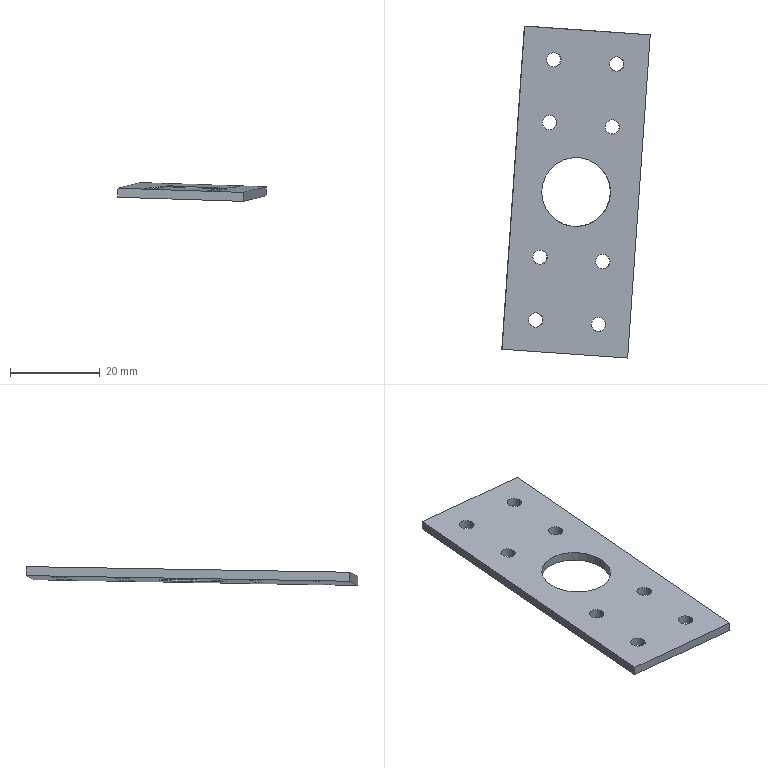Part | SolidWorks | features BaseBody 1 | 1 solid | 24 faces | box 33.003 x 73.785 x 4.177 mm | volume 3535 mm3 | cylinder 18 | plane 6 | commonest cylinder face diameters 3.2 x16 15.3 x2
STEP:
#1=CARTESIAN_POINT('',(-574.373,37.111,24.731));
#2=VERTEX_POINT('',#1);
#3=CARTESIAN_POINT('',(-571.174,37.111,24.63));
#4=VERTEX_POINT('',#3);
#5=CARTESIAN_POINT('',(-572.773,37.111,24.68));
#6=DIRECTION('',(0.03175,-0.01966,0.9993));
#7=DIRECTION('',(-0.9995,0.,0.03176));
#8=AXIS2_PLACEMENT_3D('',#5,#6,#7);
#9=CIRCLE('',#8,1.6);
#10=EDGE_CURVE('',#2,#4,#9,.T.);
#11=ORIENTED_EDGE('',*,*,#10,.T.);
#12=CARTESIAN_POINT('',(-571.238,37.15,22.631));
#13=VERTEX_POINT('',#12);
#14=CARTESIAN_POINT('',(-571.174,37.111,24.63));
#15=DIRECTION('',(-0.03175,0.01966,-0.9993));
#16=VECTOR('',#15,1000.);
#17=LINE('',#14,#16);
#18=EDGE_CURVE('',#4,#13,#17,.T.);
#19=ORIENTED_EDGE('',*,*,#18,.T.);
#20=CARTESIAN_POINT('',(-574.436,37.15,22.733));
#21=VERTEX_POINT('',#20);
#22=CARTESIAN_POINT('',(-572.837,37.15,22.682));
#23=DIRECTION('',(-0.03175,0.01966,-0.9993));
#24=DIRECTION('',(-0.9995,0.,0.03176));
#25=AXIS2_PLACEMENT_3D('',#22,#23,#24);
#26=CIRCLE('',#25,1.6);
#27=EDGE_CURVE('',#13,#21,#26,.T.);
#28=ORIENTED_EDGE('',*,*,#27,.T.);
#29=CARTESIAN_POINT('',(-574.373,37.111,24.731));
#30=DIRECTION('',(-0.03175,0.01966,-0.9993));
#31=VECTOR('',#30,1000.);
#32=LINE('',#29,#31);
#33=EDGE_CURVE('',#2,#21,#32,.T.);
#34=ORIENTED_EDGE('',*,*,#33,.F.);
#35=EDGE_LOOP('',(#11,#19,#28,#34));
#36=FACE_OUTER_BOUND('',#35,.T.);
#37=CARTESIAN_POINT('',(-572.773,37.111,24.68));
#38=DIRECTION('',(-0.03175,0.01966,-0.9993));
#39=DIRECTION('',(-0.9995,0.,0.03176));
#40=AXIS2_PLACEMENT_3D('',#37,#38,#39);
#41=CYLINDRICAL_SURFACE('',#40,1.6);
#42=ADVANCED_FACE('',(#36),#41,.F.);
#43=CARTESIAN_POINT('',(-572.151,23.147,24.386));
#44=VERTEX_POINT('',#43);
#45=CARTESIAN_POINT('',(-575.349,23.147,24.488));
#46=VERTEX_POINT('',#45);
#47=CARTESIAN_POINT('',(-573.75,23.147,24.437));
#48=DIRECTION('',(-0.03175,0.01966,-0.9993));
#49=DIRECTION('',(-0.9995,0.,0.03176));
#50=AXIS2_PLACEMENT_3D('',#47,#48,#49);
#51=CIRCLE('',#50,1.6);
#52=EDGE_CURVE('',#44,#46,#51,.T.);
#53=ORIENTED_EDGE('',*,*,#52,.F.);
#54=CARTESIAN_POINT('',(-572.214,23.186,22.387));
#55=VERTEX_POINT('',#54);
#56=CARTESIAN_POINT('',(-572.151,23.147,24.386));
#57=DIRECTION('',(-0.03175,0.01966,-0.9993));
#58=VECTOR('',#57,1000.);
#59=LINE('',#56,#58);
#60=EDGE_CURVE('',#44,#55,#59,.T.);
#61=ORIENTED_EDGE('',*,*,#60,.T.);
#62=CARTESIAN_POINT('',(-575.413,23.186,22.489));
#63=VERTEX_POINT('',#62);
#64=CARTESIAN_POINT('',(-573.813,23.186,22.438));
#65=DIRECTION('',(-0.03175,0.01966,-0.9993));
#66=DIRECTION('',(-0.9995,0.,0.03176));
#67=AXIS2_PLACEMENT_3D('',#64,#65,#66);
#68=CIRCLE('',#67,1.6);
#69=EDGE_CURVE('',#55,#63,#68,.T.);
#70=ORIENTED_EDGE('',*,*,#69,.T.);
#71=CARTESIAN_POINT('',(-575.349,23.147,24.488));
#72=DIRECTION('',(-0.03175,0.01966,-0.9993));
#73=VECTOR('',#72,1000.);
#74=LINE('',#71,#73);
#75=EDGE_CURVE('',#46,#63,#74,.T.);
#76=ORIENTED_EDGE('',*,*,#75,.F.);
#77=EDGE_LOOP('',(#53,#61,#70,#76));
#78=FACE_OUTER_BOUND('',#77,.T.);
#79=CARTESIAN_POINT('',(-573.75,23.147,24.437));
#80=DIRECTION('',(-0.03175,0.01966,-0.9993));
#81=DIRECTION('',(-0.9995,0.,0.03176));
#82=AXIS2_PLACEMENT_3D('',#79,#80,#81);
#83=CYLINDRICAL_SURFACE('',#82,1.6);
#84=ADVANCED_FACE('',(#78),#83,.F.);
#85=CARTESIAN_POINT('',(-555.123,66.061,24.689));
#86=VERTEX_POINT('',#85);
#87=CARTESIAN_POINT('',(-558.321,66.061,24.791));
#88=VERTEX_POINT('',#87);
#89=CARTESIAN_POINT('',(-556.722,66.061,24.74));
#90=DIRECTION('',(-0.03175,0.01966,-0.9993));
#91=DIRECTION('',(-0.9995,0.,0.03176));
#92=AXIS2_PLACEMENT_3D('',#89,#90,#91);
#93=CIRCLE('',#92,1.6);
#94=EDGE_CURVE('',#86,#88,#93,.T.);
#95=ORIENTED_EDGE('',*,*,#94,.F.);
#96=CARTESIAN_POINT('',(-555.186,66.1,22.691));
#97=VERTEX_POINT('',#96);
#98=CARTESIAN_POINT('',(-555.123,66.061,24.689));
#99=DIRECTION('',(-0.03175,0.01966,-0.9993));
#100=VECTOR('',#99,1000.);
#101=LINE('',#98,#100);
#102=EDGE_CURVE('',#86,#97,#101,.T.);
#103=ORIENTED_EDGE('',*,*,#102,.T.);
#104=CARTESIAN_POINT('',(-558.385,66.1,22.792));
#105=VERTEX_POINT('',#104);
#106=CARTESIAN_POINT('',(-556.786,66.1,22.741));
#107=DIRECTION('',(-0.03175,0.01966,-0.9993));
#108=DIRECTION('',(-0.9995,0.,0.03176));
#109=AXIS2_PLACEMENT_3D('',#106,#107,#108);
#110=CIRCLE('',#109,1.6);
#111=EDGE_CURVE('',#97,#105,#110,.T.);
#112=ORIENTED_EDGE('',*,*,#111,.T.);
#113=CARTESIAN_POINT('',(-558.321,66.061,24.791));
#114=DIRECTION('',(-0.03175,0.01966,-0.9993));
#115=VECTOR('',#114,1000.);
#116=LINE('',#113,#115);
#117=EDGE_CURVE('',#88,#105,#116,.T.);
#118=ORIENTED_EDGE('',*,*,#117,.F.);
#119=EDGE_LOOP('',(#95,#103,#112,#118));
#120=FACE_OUTER_BOUND('',#119,.T.);
#121=CARTESIAN_POINT('',(-556.722,66.061,24.74));
#122=DIRECTION('',(-0.03175,0.01966,-0.9993));
#123=DIRECTION('',(-0.9995,0.,0.03176));
#124=AXIS2_PLACEMENT_3D('',#121,#122,#123);
#125=CYLINDRICAL_SURFACE('',#124,1.6);
#126=ADVANCED_FACE('',(#120),#125,.F.);
#127=CARTESIAN_POINT('',(-569.082,67.029,25.152));
#128=VERTEX_POINT('',#127);
#129=CARTESIAN_POINT('',(-572.28,67.029,25.253));
#130=VERTEX_POINT('',#129);
#131=CARTESIAN_POINT('',(-570.681,67.029,25.203));
#132=DIRECTION('',(-0.03175,0.01966,-0.9993));
#133=DIRECTION('',(-0.9995,0.,0.03176));
#134=AXIS2_PLACEMENT_3D('',#131,#132,#133);
#135=CIRCLE('',#134,1.6);
#136=EDGE_CURVE('',#128,#130,#135,.T.);
#137=ORIENTED_EDGE('',*,*,#136,.F.);
#138=CARTESIAN_POINT('',(-569.145,67.068,23.153));
#139=VERTEX_POINT('',#138);
#140=CARTESIAN_POINT('',(-569.082,67.029,25.152));
#141=DIRECTION('',(-0.03175,0.01966,-0.9993));
#142=VECTOR('',#141,1000.);
#143=LINE('',#140,#142);
#144=EDGE_CURVE('',#128,#139,#143,.T.);
#145=ORIENTED_EDGE('',*,*,#144,.T.);
#146=CARTESIAN_POINT('',(-572.344,67.068,23.255));
#147=VERTEX_POINT('',#146);
#148=CARTESIAN_POINT('',(-570.745,67.068,23.204));
#149=DIRECTION('',(-0.03175,0.01966,-0.9993));
#150=DIRECTION('',(-0.9995,0.,0.03176));
#151=AXIS2_PLACEMENT_3D('',#148,#149,#150);
#152=CIRCLE('',#151,1.6);
#153=EDGE_CURVE('',#139,#147,#152,.T.);
#154=ORIENTED_EDGE('',*,*,#153,.T.);
#155=CARTESIAN_POINT('',(-572.28,67.029,25.253));
#156=DIRECTION('',(-0.03175,0.01966,-0.9993));
#157=VECTOR('',#156,1000.);
#158=LINE('',#155,#157);
#159=EDGE_CURVE('',#130,#147,#158,.T.);
#160=ORIENTED_EDGE('',*,*,#159,.F.);
#161=EDGE_LOOP('',(#137,#145,#154,#160));
#162=FACE_OUTER_BOUND('',#161,.T.);
#163=CARTESIAN_POINT('',(-570.681,67.029,25.203));
#164=DIRECTION('',(-0.03175,0.01966,-0.9993));
#165=DIRECTION('',(-0.9995,0.,0.03176));
#166=AXIS2_PLACEMENT_3D('',#163,#164,#165);
#167=CYLINDRICAL_SURFACE('',#166,1.6);
#168=ADVANCED_FACE('',(#162),#167,.F.);
#169=CARTESIAN_POINT('',(-568.105,80.992,25.396));
#170=VERTEX_POINT('',#169);
#171=CARTESIAN_POINT('',(-571.304,80.992,25.497));
#172=VERTEX_POINT('',#171);
#173=CARTESIAN_POINT('',(-569.704,80.992,25.446));
#174=DIRECTION('',(-0.03175,0.01966,-0.9993));
#175=DIRECTION('',(-0.9995,0.,0.03176));
#176=AXIS2_PLACEMENT_3D('',#173,#174,#175);
#177=CIRCLE('',#176,1.6);
#178=EDGE_CURVE('',#170,#172,#177,.T.);
#179=ORIENTED_EDGE('',*,*,#178,.F.);
#180=CARTESIAN_POINT('',(-568.169,81.032,23.397));
#181=VERTEX_POINT('',#180);
#182=CARTESIAN_POINT('',(-568.105,80.992,25.396));
#183=DIRECTION('',(-0.03175,0.01966,-0.9993));
#184=VECTOR('',#183,1000.);
#185=LINE('',#182,#184);
#186=EDGE_CURVE('',#170,#181,#185,.T.);
#187=ORIENTED_EDGE('',*,*,#186,.T.);
#188=CARTESIAN_POINT('',(-571.367,81.032,23.499));
#189=VERTEX_POINT('',#188);
#190=CARTESIAN_POINT('',(-569.768,81.032,23.448));
#191=DIRECTION('',(-0.03175,0.01966,-0.9993));
#192=DIRECTION('',(-0.9995,0.,0.03176));
#193=AXIS2_PLACEMENT_3D('',#190,#191,#192);
#194=CIRCLE('',#193,1.6);
#195=EDGE_CURVE('',#181,#189,#194,.T.);
#196=ORIENTED_EDGE('',*,*,#195,.T.);
#197=CARTESIAN_POINT('',(-571.304,80.992,25.497));
#198=DIRECTION('',(-0.03175,0.01966,-0.9993));
#199=VECTOR('',#198,1000.);
#200=LINE('',#197,#199);
#201=EDGE_CURVE('',#172,#189,#200,.T.);
#202=ORIENTED_EDGE('',*,*,#201,.F.);
#203=EDGE_LOOP('',(#179,#187,#196,#202));
#204=FACE_OUTER_BOUND('',#203,.T.);
#205=CARTESIAN_POINT('',(-569.704,80.992,25.446));
#206=DIRECTION('',(-0.03175,0.01966,-0.9993));
#207=DIRECTION('',(-0.9995,0.,0.03176));
#208=AXIS2_PLACEMENT_3D('',#205,#206,#207);
#209=CYLINDRICAL_SURFACE('',#208,1.6);
#210=ADVANCED_FACE('',(#204),#209,.F.);
#211=CARTESIAN_POINT('',(-554.146,80.024,24.933));
#212=VERTEX_POINT('',#211);
#213=CARTESIAN_POINT('',(-557.345,80.024,25.035));
#214=VERTEX_POINT('',#213);
#215=CARTESIAN_POINT('',(-555.746,80.024,24.984));
#216=DIRECTION('',(-0.03175,0.01966,-0.9993));
#217=DIRECTION('',(-0.9995,0.,0.03176));
#218=AXIS2_PLACEMENT_3D('',#215,#216,#217);
#219=CIRCLE('',#218,1.6);
#220=EDGE_CURVE('',#212,#214,#219,.T.);
#221=ORIENTED_EDGE('',*,*,#220,.F.);
#222=CARTESIAN_POINT('',(-554.21,80.064,22.934));
#223=VERTEX_POINT('',#222);
#224=CARTESIAN_POINT('',(-554.146,80.024,24.933));
#225=DIRECTION('',(-0.03175,0.01966,-0.9993));
#226=VECTOR('',#225,1000.);
#227=LINE('',#224,#226);
#228=EDGE_CURVE('',#212,#223,#227,.T.);
#229=ORIENTED_EDGE('',*,*,#228,.T.);
#230=CARTESIAN_POINT('',(-557.408,80.064,23.036));
#231=VERTEX_POINT('',#230);
#232=CARTESIAN_POINT('',(-555.809,80.064,22.985));
#233=DIRECTION('',(-0.03175,0.01966,-0.9993));
#234=DIRECTION('',(-0.9995,0.,0.03176));
#235=AXIS2_PLACEMENT_3D('',#232,#233,#234);
#236=CIRCLE('',#235,1.6);
#237=EDGE_CURVE('',#223,#231,#236,.T.);
#238=ORIENTED_EDGE('',*,*,#237,.T.);
#239=CARTESIAN_POINT('',(-557.345,80.024,25.035));
#240=DIRECTION('',(-0.03175,0.01966,-0.9993));
#241=VECTOR('',#240,1000.);
#242=LINE('',#239,#241);
#243=EDGE_CURVE('',#214,#231,#242,.T.);
#244=ORIENTED_EDGE('',*,*,#243,.F.);
#245=EDGE_LOOP('',(#221,#229,#238,#244));
#246=FACE_OUTER_BOUND('',#245,.T.);
#247=CARTESIAN_POINT('',(-555.746,80.024,24.984));
#248=DIRECTION('',(-0.03175,0.01966,-0.9993));
#249=DIRECTION('',(-0.9995,0.,0.03176));
#250=AXIS2_PLACEMENT_3D('',#247,#248,#249);
#251=CYLINDRICAL_SURFACE('',#250,1.6);
#252=ADVANCED_FACE('',(#246),#251,.F.);
#253=CARTESIAN_POINT('',(-557.102,51.586,24.467));
#254=VERTEX_POINT('',#253);
#255=CARTESIAN_POINT('',(-572.394,51.586,24.953));
#256=VERTEX_POINT('',#255);
#257=CARTESIAN_POINT('',(-564.748,51.586,24.71));
#258=DIRECTION('',(-0.03175,0.01966,-0.9993));
#259=DIRECTION('',(-0.9995,0.,0.03176));
#260=AXIS2_PLACEMENT_3D('',#257,#258,#259);
#261=CIRCLE('',#260,7.65);
#262=EDGE_CURVE('',#254,#256,#261,.T.);
#263=ORIENTED_EDGE('',*,*,#262,.F.);
#264=CARTESIAN_POINT('',(-557.165,51.625,22.469));
#265=VERTEX_POINT('',#264);
#266=CARTESIAN_POINT('',(-557.102,51.586,24.467));
#267=DIRECTION('',(-0.03175,0.01966,-0.9993));
#268=VECTOR('',#267,1000.);
#269=LINE('',#266,#268);
#270=EDGE_CURVE('',#254,#265,#269,.T.);
#271=ORIENTED_EDGE('',*,*,#270,.T.);
#272=CARTESIAN_POINT('',(-572.457,51.625,22.955));
#273=VERTEX_POINT('',#272);
#274=CARTESIAN_POINT('',(-564.811,51.625,22.712));
#275=DIRECTION('',(-0.03175,0.01966,-0.9993));
#276=DIRECTION('',(-0.9995,0.,0.03176));
#277=AXIS2_PLACEMENT_3D('',#274,#275,#276);
#278=CIRCLE('',#277,7.65);
#279=EDGE_CURVE('',#265,#273,#278,.T.);
#280=ORIENTED_EDGE('',*,*,#279,.T.);
#281=CARTESIAN_POINT('',(-572.394,51.586,24.953));
#282=DIRECTION('',(-0.03175,0.01966,-0.9993));
#283=VECTOR('',#282,1000.);
#284=LINE('',#281,#283);
#285=EDGE_CURVE('',#256,#273,#284,.T.);
#286=ORIENTED_EDGE('',*,*,#285,.F.);
#287=EDGE_LOOP('',(#263,#271,#280,#286));
#288=FACE_OUTER_BOUND('',#287,.T.);
#289=CARTESIAN_POINT('',(-564.748,51.586,24.71));
#290=DIRECTION('',(-0.03175,0.01966,-0.9993));
#291=DIRECTION('',(-0.9995,0.,0.03176));
#292=AXIS2_PLACEMENT_3D('',#289,#290,#291);
#293=CYLINDRICAL_SURFACE('',#292,7.65);
#294=ADVANCED_FACE('',(#288),#293,.F.);
#295=CARTESIAN_POINT('',(-558.192,22.179,23.923));
#296=VERTEX_POINT('',#295);
#297=CARTESIAN_POINT('',(-561.39,22.179,24.025));
#298=VERTEX_POINT('',#297);
#299=CARTESIAN_POINT('',(-559.791,22.179,23.974));
#300=DIRECTION('',(-0.03175,0.01966,-0.9993));
#301=DIRECTION('',(-0.9995,0.,0.03176));
#302=AXIS2_PLACEMENT_3D('',#299,#300,#301);
#303=CIRCLE('',#302,1.6);
#304=EDGE_CURVE('',#296,#298,#303,.T.);
#305=ORIENTED_EDGE('',*,*,#304,.F.);
#306=CARTESIAN_POINT('',(-558.255,22.218,21.925));
#307=VERTEX_POINT('',#306);
#308=CARTESIAN_POINT('',(-558.192,22.179,23.923));
#309=DIRECTION('',(-0.03175,0.01966,-0.9993));
#310=VECTOR('',#309,1000.);
#311=LINE('',#308,#310);
#312=EDGE_CURVE('',#296,#307,#311,.T.);
#313=ORIENTED_EDGE('',*,*,#312,.T.);
#314=CARTESIAN_POINT('',(-561.454,22.218,22.026));
#315=VERTEX_POINT('',#314);
#316=CARTESIAN_POINT('',(-559.855,22.218,21.976));
#317=DIRECTION('',(-0.03175,0.01966,-0.9993));
#318=DIRECTION('',(-0.9995,0.,0.03176));
#319=AXIS2_PLACEMENT_3D('',#316,#317,#318);
#320=CIRCLE('',#319,1.6);
#321=EDGE_CURVE('',#307,#315,#320,.T.);
#322=ORIENTED_EDGE('',*,*,#321,.T.);
#323=CARTESIAN_POINT('',(-561.39,22.179,24.025));
#324=DIRECTION('',(-0.03175,0.01966,-0.9993));
#325=VECTOR('',#324,1000.);
#326=LINE('',#323,#325);
#327=EDGE_CURVE('',#298,#315,#326,.T.);
#328=ORIENTED_EDGE('',*,*,#327,.F.);
#329=EDGE_LOOP('',(#305,#313,#322,#328));
#330=FACE_OUTER_BOUND('',#329,.T.);
#331=CARTESIAN_POINT('',(-559.791,22.179,23.974));
#332=DIRECTION('',(-0.03175,0.01966,-0.9993));
#333=DIRECTION('',(-0.9995,0.,0.03176));
#334=AXIS2_PLACEMENT_3D('',#331,#332,#333);
#335=CYLINDRICAL_SURFACE('',#334,1.6);
#336=ADVANCED_FACE('',(#330),#335,.F.);
#337=CARTESIAN_POINT('',(-557.215,36.143,24.167));
#338=VERTEX_POINT('',#337);
#339=CARTESIAN_POINT('',(-560.414,36.143,24.269));
#340=VERTEX_POINT('',#339);
#341=CARTESIAN_POINT('',(-558.815,36.143,24.218));
#342=DIRECTION('',(-0.03175,0.01966,-0.9993));
#343=DIRECTION('',(-0.9995,0.,0.03176));
#344=AXIS2_PLACEMENT_3D('',#341,#342,#343);
#345=CIRCLE('',#344,1.6);
#346=EDGE_CURVE('',#338,#340,#345,.T.);
#347=ORIENTED_EDGE('',*,*,#346,.F.);
#348=CARTESIAN_POINT('',(-557.279,36.182,22.168));
#349=VERTEX_POINT('',#348);
#350=CARTESIAN_POINT('',(-557.215,36.143,24.167));
#351=DIRECTION('',(-0.03175,0.01966,-0.9993));
#352=VECTOR('',#351,1000.);
#353=LINE('',#350,#352);
#354=EDGE_CURVE('',#338,#349,#353,.T.);
#355=ORIENTED_EDGE('',*,*,#354,.T.);
#356=CARTESIAN_POINT('',(-560.477,36.182,22.27));
#357=VERTEX_POINT('',#356);
#358=CARTESIAN_POINT('',(-558.878,36.182,22.219));
#359=DIRECTION('',(-0.03175,0.01966,-0.9993));
#360=DIRECTION('',(-0.9995,0.,0.03176));
#361=AXIS2_PLACEMENT_3D('',#358,#359,#360);
#362=CIRCLE('',#361,1.6);
#363=EDGE_CURVE('',#349,#357,#362,.T.);
#364=ORIENTED_EDGE('',*,*,#363,.T.);
#365=CARTESIAN_POINT('',(-560.414,36.143,24.269));
#366=DIRECTION('',(-0.03175,0.01966,-0.9993));
#367=VECTOR('',#366,1000.);
#368=LINE('',#365,#367);
#369=EDGE_CURVE('',#340,#357,#368,.T.);
#370=ORIENTED_EDGE('',*,*,#369,.F.);
#371=EDGE_LOOP('',(#347,#355,#364,#370));
#372=FACE_OUTER_BOUND('',#371,.T.);
#373=CARTESIAN_POINT('',(-558.815,36.143,24.218));
#374=DIRECTION('',(-0.03175,0.01966,-0.9993));
#375=DIRECTION('',(-0.9995,0.,0.03176));
#376=AXIS2_PLACEMENT_3D('',#373,#374,#375);
#377=CYLINDRICAL_SURFACE('',#376,1.6);
#378=ADVANCED_FACE('',(#372),#377,.F.);
#379=ORIENTED_EDGE('',*,*,#18,.F.);
#380=CARTESIAN_POINT('',(-572.773,37.111,24.68));
#381=DIRECTION('',(0.03175,-0.01966,0.9993));
#382=DIRECTION('',(-0.9995,0.,0.03176));
#383=AXIS2_PLACEMENT_3D('',#380,#381,#382);
#384=CIRCLE('',#383,1.6);
#385=EDGE_CURVE('',#4,#2,#384,.T.);
#386=ORIENTED_EDGE('',*,*,#385,.T.);
#387=ORIENTED_EDGE('',*,*,#33,.T.);
#388=CARTESIAN_POINT('',(-572.837,37.15,22.682));
#389=DIRECTION('',(-0.03175,0.01966,-0.9993));
#390=DIRECTION('',(-0.9995,0.,0.03176));
#391=AXIS2_PLACEMENT_3D('',#388,#389,#390);
#392=CIRCLE('',#391,1.6);
#393=EDGE_CURVE('',#21,#13,#392,.T.);
#394=ORIENTED_EDGE('',*,*,#393,.T.);
#395=EDGE_LOOP('',(#379,#386,#387,#394));
#396=FACE_OUTER_BOUND('',#395,.T.);
#397=CARTESIAN_POINT('',(-572.773,37.111,24.68));
#398=DIRECTION('',(-0.03175,0.01966,-0.9993));
#399=DIRECTION('',(-0.9995,0.,0.03176));
#400=AXIS2_PLACEMENT_3D('',#397,#398,#399);
#401=CYLINDRICAL_SURFACE('',#400,1.6);
#402=ADVANCED_FACE('',(#396),#401,.F.);
#403=ORIENTED_EDGE('',*,*,#393,.F.);
#404=ORIENTED_EDGE('',*,*,#27,.F.);
#405=EDGE_LOOP('',(#403,#404));
#406=FACE_BOUND('',#405,.T.);
#407=CARTESIAN_POINT('',(-573.813,23.186,22.438));
#408=DIRECTION('',(-0.03175,0.01966,-0.9993));
#409=DIRECTION('',(-0.9995,0.,0.03176));
#410=AXIS2_PLACEMENT_3D('',#407,#408,#409);
#411=CIRCLE('',#410,1.6);
#412=EDGE_CURVE('',#63,#55,#411,.T.);
#413=ORIENTED_EDGE('',*,*,#412,.F.);
#414=ORIENTED_EDGE('',*,*,#69,.F.);
#415=EDGE_LOOP('',(#413,#414));
#416=FACE_BOUND('',#415,.T.);
#417=CARTESIAN_POINT('',(-556.786,66.1,22.741));
#418=DIRECTION('',(-0.03175,0.01966,-0.9993));
#419=DIRECTION('',(-0.9995,0.,0.03176));
#420=AXIS2_PLACEMENT_3D('',#417,#418,#419);
#421=CIRCLE('',#420,1.6);
#422=EDGE_CURVE('',#105,#97,#421,.T.);
#423=ORIENTED_EDGE('',*,*,#422,.F.);
#424=ORIENTED_EDGE('',*,*,#111,.F.);
#425=EDGE_LOOP('',(#423,#424));
#426=FACE_BOUND('',#425,.T.);
#427=CARTESIAN_POINT('',(-570.745,67.068,23.204));
#428=DIRECTION('',(-0.03175,0.01966,-0.9993));
#429=DIRECTION('',(-0.9995,0.,0.03176));
#430=AXIS2_PLACEMENT_3D('',#427,#428,#429);
#431=CIRCLE('',#430,1.6);
#432=EDGE_CURVE('',#147,#139,#431,.T.);
#433=ORIENTED_EDGE('',*,*,#432,.F.);
#434=ORIENTED_EDGE('',*,*,#153,.F.);
#435=EDGE_LOOP('',(#433,#434));
#436=FACE_BOUND('',#435,.T.);
#437=CARTESIAN_POINT('',(-569.768,81.032,23.448));
#438=DIRECTION('',(-0.03175,0.01966,-0.9993));
#439=DIRECTION('',(-0.9995,0.,0.03176));
#440=AXIS2_PLACEMENT_3D('',#437,#438,#439);
#441=CIRCLE('',#440,1.6);
#442=EDGE_CURVE('',#189,#181,#441,.T.);
#443=ORIENTED_EDGE('',*,*,#442,.F.);
#444=ORIENTED_EDGE('',*,*,#195,.F.);
#445=EDGE_LOOP('',(#443,#444));
#446=FACE_BOUND('',#445,.T.);
#447=CARTESIAN_POINT('',(-555.809,80.064,22.985));
#448=DIRECTION('',(-0.03175,0.01966,-0.9993));
#449=DIRECTION('',(-0.9995,0.,0.03176));
#450=AXIS2_PLACEMENT_3D('',#447,#448,#449);
#451=CIRCLE('',#450,1.6);
#452=EDGE_CURVE('',#231,#223,#451,.T.);
#453=ORIENTED_EDGE('',*,*,#452,.F.);
#454=ORIENTED_EDGE('',*,*,#237,.F.);
#455=EDGE_LOOP('',(#453,#454));
#456=FACE_BOUND('',#455,.T.);
#457=CARTESIAN_POINT('',(-564.811,51.625,22.712));
#458=DIRECTION('',(-0.03175,0.01966,-0.9993));
#459=DIRECTION('',(-0.9995,0.,0.03176));
#460=AXIS2_PLACEMENT_3D('',#457,#458,#459);
#461=CIRCLE('',#460,7.65);
#462=EDGE_CURVE('',#273,#265,#461,.T.);
#463=ORIENTED_EDGE('',*,*,#462,.F.);
#464=ORIENTED_EDGE('',*,*,#279,.F.);
#465=EDGE_LOOP('',(#463,#464));
#466=FACE_BOUND('',#465,.T.);
#467=CARTESIAN_POINT('',(-559.855,22.218,21.976));
#468=DIRECTION('',(-0.03175,0.01966,-0.9993));
#469=DIRECTION('',(-0.9995,0.,0.03176));
#470=AXIS2_PLACEMENT_3D('',#467,#468,#469);
#471=CIRCLE('',#470,1.6);
#472=EDGE_CURVE('',#315,#307,#471,.T.);
#473=ORIENTED_EDGE('',*,*,#472,.F.);
#474=ORIENTED_EDGE('',*,*,#321,.F.);
#475=EDGE_LOOP('',(#473,#474));
#476=FACE_BOUND('',#475,.T.);
#477=CARTESIAN_POINT('',(-558.878,36.182,22.219));
#478=DIRECTION('',(-0.03175,0.01966,-0.9993));
#479=DIRECTION('',(-0.9995,0.,0.03176));
#480=AXIS2_PLACEMENT_3D('',#477,#478,#479);
#481=CIRCLE('',#480,1.6);
#482=EDGE_CURVE('',#357,#349,#481,.T.);
#483=ORIENTED_EDGE('',*,*,#482,.F.);
#484=ORIENTED_EDGE('',*,*,#363,.F.);
#485=EDGE_LOOP('',(#483,#484));
#486=FACE_BOUND('',#485,.T.);
#487=CARTESIAN_POINT('',(-548.341,86.561,22.876));
#488=VERTEX_POINT('',#487);
#489=CARTESIAN_POINT('',(-576.259,88.498,23.801));
#490=VERTEX_POINT('',#489);
#491=CARTESIAN_POINT('',(-548.341,86.561,22.876));
#492=DIRECTION('',(-0.9971,0.06916,0.03304));
#493=VECTOR('',#492,1000.);
#494=LINE('',#491,#493);
#495=EDGE_CURVE('',#488,#490,#494,.T.);
#496=ORIENTED_EDGE('',*,*,#495,.F.);
#497=CARTESIAN_POINT('',(-553.364,14.752,21.622));
#498=VERTEX_POINT('',#497);
#499=CARTESIAN_POINT('',(-553.364,14.752,21.622));
#500=DIRECTION('',(0.06976,0.9974,0.01741));
#501=VECTOR('',#500,1000.);
#502=LINE('',#499,#501);
#503=EDGE_CURVE('',#498,#488,#502,.T.);
#504=ORIENTED_EDGE('',*,*,#503,.F.);
#505=CARTESIAN_POINT('',(-581.281,16.689,22.548));
#506=VERTEX_POINT('',#505);
#507=CARTESIAN_POINT('',(-581.281,16.689,22.548));
#508=DIRECTION('',(0.9971,-0.06916,-0.03304));
#509=VECTOR('',#508,1000.);
#510=LINE('',#507,#509);
#511=EDGE_CURVE('',#506,#498,#510,.T.);
#512=ORIENTED_EDGE('',*,*,#511,.F.);
#513=CARTESIAN_POINT('',(-576.259,88.498,23.801));
#514=DIRECTION('',(-0.06976,-0.9974,-0.01741));
#515=VECTOR('',#514,1000.);
#516=LINE('',#513,#515);
#517=EDGE_CURVE('',#490,#506,#516,.T.);
#518=ORIENTED_EDGE('',*,*,#517,.F.);
#519=EDGE_LOOP('',(#496,#504,#512,#518));
#520=FACE_OUTER_BOUND('',#519,.T.);
#521=CARTESIAN_POINT('',(-581.48,14.31,22.507));
#522=DIRECTION('',(0.03175,-0.01966,0.9993));
#523=DIRECTION('',(0.9995,0.,-0.03176));
#524=AXIS2_PLACEMENT_3D('',#521,#522,#523);
#525=PLANE('',#524);
#526=ADVANCED_FACE('',(#406,#416,#426,#436,#446,#456,#466,#476,#486,#520),#525,.F.);
#527=ORIENTED_EDGE('',*,*,#10,.F.);
#528=ORIENTED_EDGE('',*,*,#385,.F.);
#529=EDGE_LOOP('',(#527,#528));
#530=FACE_BOUND('',#529,.T.);
#531=CARTESIAN_POINT('',(-573.75,23.147,24.437));
#532=DIRECTION('',(-0.03175,0.01966,-0.9993));
#533=DIRECTION('',(-0.9995,0.,0.03176));
#534=AXIS2_PLACEMENT_3D('',#531,#532,#533);
#535=CIRCLE('',#534,1.6);
#536=EDGE_CURVE('',#46,#44,#535,.T.);
#537=ORIENTED_EDGE('',*,*,#536,.T.);
#538=ORIENTED_EDGE('',*,*,#52,.T.);
#539=EDGE_LOOP('',(#537,#538));
#540=FACE_BOUND('',#539,.T.);
#541=CARTESIAN_POINT('',(-556.722,66.061,24.74));
#542=DIRECTION('',(-0.03175,0.01966,-0.9993));
#543=DIRECTION('',(-0.9995,0.,0.03176));
#544=AXIS2_PLACEMENT_3D('',#541,#542,#543);
#545=CIRCLE('',#544,1.6);
#546=EDGE_CURVE('',#88,#86,#545,.T.);
#547=ORIENTED_EDGE('',*,*,#546,.T.);
#548=ORIENTED_EDGE('',*,*,#94,.T.);
#549=EDGE_LOOP('',(#547,#548));
#550=FACE_BOUND('',#549,.T.);
#551=CARTESIAN_POINT('',(-570.681,67.029,25.203));
#552=DIRECTION('',(-0.03175,0.01966,-0.9993));
#553=DIRECTION('',(-0.9995,0.,0.03176));
#554=AXIS2_PLACEMENT_3D('',#551,#552,#553);
#555=CIRCLE('',#554,1.6);
#556=EDGE_CURVE('',#130,#128,#555,.T.);
#557=ORIENTED_EDGE('',*,*,#556,.T.);
#558=ORIENTED_EDGE('',*,*,#136,.T.);
#559=EDGE_LOOP('',(#557,#558));
#560=FACE_BOUND('',#559,.T.);
#561=CARTESIAN_POINT('',(-569.704,80.992,25.446));
#562=DIRECTION('',(-0.03175,0.01966,-0.9993));
#563=DIRECTION('',(-0.9995,0.,0.03176));
#564=AXIS2_PLACEMENT_3D('',#561,#562,#563);
#565=CIRCLE('',#564,1.6);
#566=EDGE_CURVE('',#172,#170,#565,.T.);
#567=ORIENTED_EDGE('',*,*,#566,.T.);
#568=ORIENTED_EDGE('',*,*,#178,.T.);
#569=EDGE_LOOP('',(#567,#568));
#570=FACE_BOUND('',#569,.T.);
#571=CARTESIAN_POINT('',(-555.746,80.024,24.984));
#572=DIRECTION('',(-0.03175,0.01966,-0.9993));
#573=DIRECTION('',(-0.9995,0.,0.03176));
#574=AXIS2_PLACEMENT_3D('',#571,#572,#573);
#575=CIRCLE('',#574,1.6);
#576=EDGE_CURVE('',#214,#212,#575,.T.);
#577=ORIENTED_EDGE('',*,*,#576,.T.);
#578=ORIENTED_EDGE('',*,*,#220,.T.);
#579=EDGE_LOOP('',(#577,#578));
#580=FACE_BOUND('',#579,.T.);
#581=CARTESIAN_POINT('',(-564.748,51.586,24.71));
#582=DIRECTION('',(-0.03175,0.01966,-0.9993));
#583=DIRECTION('',(-0.9995,0.,0.03176));
#584=AXIS2_PLACEMENT_3D('',#581,#582,#583);
#585=CIRCLE('',#584,7.65);
#586=EDGE_CURVE('',#256,#254,#585,.T.);
#587=ORIENTED_EDGE('',*,*,#586,.T.);
#588=ORIENTED_EDGE('',*,*,#262,.T.);
#589=EDGE_LOOP('',(#587,#588));
#590=FACE_BOUND('',#589,.T.);
#591=CARTESIAN_POINT('',(-559.791,22.179,23.974));
#592=DIRECTION('',(-0.03175,0.01966,-0.9993));
#593=DIRECTION('',(-0.9995,0.,0.03176));
#594=AXIS2_PLACEMENT_3D('',#591,#592,#593);
#595=CIRCLE('',#594,1.6);
#596=EDGE_CURVE('',#298,#296,#595,.T.);
#597=ORIENTED_EDGE('',*,*,#596,.T.);
#598=ORIENTED_EDGE('',*,*,#304,.T.);
#599=EDGE_LOOP('',(#597,#598));
#600=FACE_BOUND('',#599,.T.);
#601=CARTESIAN_POINT('',(-558.815,36.143,24.218));
#602=DIRECTION('',(-0.03175,0.01966,-0.9993));
#603=DIRECTION('',(-0.9995,0.,0.03176));
#604=AXIS2_PLACEMENT_3D('',#601,#602,#603);
#605=CIRCLE('',#604,1.6);
#606=EDGE_CURVE('',#340,#338,#605,.T.);
#607=ORIENTED_EDGE('',*,*,#606,.T.);
#608=ORIENTED_EDGE('',*,*,#346,.T.);
#609=EDGE_LOOP('',(#607,#608));
#610=FACE_BOUND('',#609,.T.);
#611=CARTESIAN_POINT('',(-553.3,14.713,23.621));
#612=VERTEX_POINT('',#611);
#613=CARTESIAN_POINT('',(-548.278,86.522,24.874));
#614=VERTEX_POINT('',#613);
#615=CARTESIAN_POINT('',(-553.3,14.713,23.621));
#616=DIRECTION('',(0.06976,0.9974,0.01741));
#617=VECTOR('',#616,1000.);
#618=LINE('',#615,#617);
#619=EDGE_CURVE('',#612,#614,#618,.T.);
#620=ORIENTED_EDGE('',*,*,#619,.T.);
#621=CARTESIAN_POINT('',(-576.196,88.458,25.8));
#622=VERTEX_POINT('',#621);
#623=CARTESIAN_POINT('',(-548.278,86.522,24.874));
#624=DIRECTION('',(-0.9971,0.06916,0.03304));
#625=VECTOR('',#624,1000.);
#626=LINE('',#623,#625);
#627=EDGE_CURVE('',#614,#622,#626,.T.);
#628=ORIENTED_EDGE('',*,*,#627,.T.);
#629=CARTESIAN_POINT('',(-581.218,16.649,24.546));
#630=VERTEX_POINT('',#629);
#631=CARTESIAN_POINT('',(-576.196,88.458,25.8));
#632=DIRECTION('',(-0.06976,-0.9974,-0.01741));
#633=VECTOR('',#632,1000.);
#634=LINE('',#631,#633);
#635=EDGE_CURVE('',#622,#630,#634,.T.);
#636=ORIENTED_EDGE('',*,*,#635,.T.);
#637=CARTESIAN_POINT('',(-581.218,16.649,24.546));
#638=DIRECTION('',(0.9971,-0.06916,-0.03304));
#639=VECTOR('',#638,1000.);
#640=LINE('',#637,#639);
#641=EDGE_CURVE('',#630,#612,#640,.T.);
#642=ORIENTED_EDGE('',*,*,#641,.T.);
#643=EDGE_LOOP('',(#620,#628,#636,#642));
#644=FACE_OUTER_BOUND('',#643,.T.);
#645=CARTESIAN_POINT('',(-581.417,14.271,24.506));
#646=DIRECTION('',(0.03175,-0.01966,0.9993));
#647=DIRECTION('',(0.9995,0.,-0.03176));
#648=AXIS2_PLACEMENT_3D('',#645,#646,#647);
#649=PLANE('',#648);
#650=ADVANCED_FACE('',(#530,#540,#550,#560,#570,#580,#590,#600,#610,#644),#649,.T.);
#651=ORIENTED_EDGE('',*,*,#60,.F.);
#652=ORIENTED_EDGE('',*,*,#536,.F.);
#653=ORIENTED_EDGE('',*,*,#75,.T.);
#654=ORIENTED_EDGE('',*,*,#412,.T.);
#655=EDGE_LOOP('',(#651,#652,#653,#654));
#656=FACE_OUTER_BOUND('',#655,.T.);
#657=CARTESIAN_POINT('',(-573.75,23.147,24.437));
#658=DIRECTION('',(-0.03175,0.01966,-0.9993));
#659=DIRECTION('',(-0.9995,0.,0.03176));
#660=AXIS2_PLACEMENT_3D('',#657,#658,#659);
#661=CYLINDRICAL_SURFACE('',#660,1.6);
#662=ADVANCED_FACE('',(#656),#661,.F.);
#663=ORIENTED_EDGE('',*,*,#102,.F.);
#664=ORIENTED_EDGE('',*,*,#546,.F.);
#665=ORIENTED_EDGE('',*,*,#117,.T.);
#666=ORIENTED_EDGE('',*,*,#422,.T.);
#667=EDGE_LOOP('',(#663,#664,#665,#666));
#668=FACE_OUTER_BOUND('',#667,.T.);
#669=CARTESIAN_POINT('',(-556.722,66.061,24.74));
#670=DIRECTION('',(-0.03175,0.01966,-0.9993));
#671=DIRECTION('',(-0.9995,0.,0.03176));
#672=AXIS2_PLACEMENT_3D('',#669,#670,#671);
#673=CYLINDRICAL_SURFACE('',#672,1.6);
#674=ADVANCED_FACE('',(#668),#673,.F.);
#675=ORIENTED_EDGE('',*,*,#144,.F.);
#676=ORIENTED_EDGE('',*,*,#556,.F.);
#677=ORIENTED_EDGE('',*,*,#159,.T.);
#678=ORIENTED_EDGE('',*,*,#432,.T.);
#679=EDGE_LOOP('',(#675,#676,#677,#678));
#680=FACE_OUTER_BOUND('',#679,.T.);
#681=CARTESIAN_POINT('',(-570.681,67.029,25.203));
#682=DIRECTION('',(-0.03175,0.01966,-0.9993));
#683=DIRECTION('',(-0.9995,0.,0.03176));
#684=AXIS2_PLACEMENT_3D('',#681,#682,#683);
#685=CYLINDRICAL_SURFACE('',#684,1.6);
#686=ADVANCED_FACE('',(#680),#685,.F.);
#687=ORIENTED_EDGE('',*,*,#186,.F.);
#688=ORIENTED_EDGE('',*,*,#566,.F.);
#689=ORIENTED_EDGE('',*,*,#201,.T.);
#690=ORIENTED_EDGE('',*,*,#442,.T.);
#691=EDGE_LOOP('',(#687,#688,#689,#690));
#692=FACE_OUTER_BOUND('',#691,.T.);
#693=CARTESIAN_POINT('',(-569.704,80.992,25.446));
#694=DIRECTION('',(-0.03175,0.01966,-0.9993));
#695=DIRECTION('',(-0.9995,0.,0.03176));
#696=AXIS2_PLACEMENT_3D('',#693,#694,#695);
#697=CYLINDRICAL_SURFACE('',#696,1.6);
#698=ADVANCED_FACE('',(#692),#697,.F.);
#699=ORIENTED_EDGE('',*,*,#228,.F.);
#700=ORIENTED_EDGE('',*,*,#576,.F.);
#701=ORIENTED_EDGE('',*,*,#243,.T.);
#702=ORIENTED_EDGE('',*,*,#452,.T.);
#703=EDGE_LOOP('',(#699,#700,#701,#702));
#704=FACE_OUTER_BOUND('',#703,.T.);
#705=CARTESIAN_POINT('',(-555.746,80.024,24.984));
#706=DIRECTION('',(-0.03175,0.01966,-0.9993));
#707=DIRECTION('',(-0.9995,0.,0.03176));
#708=AXIS2_PLACEMENT_3D('',#705,#706,#707);
#709=CYLINDRICAL_SURFACE('',#708,1.6);
#710=ADVANCED_FACE('',(#704),#709,.F.);
#711=ORIENTED_EDGE('',*,*,#270,.F.);
#712=ORIENTED_EDGE('',*,*,#586,.F.);
#713=ORIENTED_EDGE('',*,*,#285,.T.);
#714=ORIENTED_EDGE('',*,*,#462,.T.);
#715=EDGE_LOOP('',(#711,#712,#713,#714));
#716=FACE_OUTER_BOUND('',#715,.T.);
#717=CARTESIAN_POINT('',(-564.748,51.586,24.71));
#718=DIRECTION('',(-0.03175,0.01966,-0.9993));
#719=DIRECTION('',(-0.9995,0.,0.03176));
#720=AXIS2_PLACEMENT_3D('',#717,#718,#719);
#721=CYLINDRICAL_SURFACE('',#720,7.65);
#722=ADVANCED_FACE('',(#716),#721,.F.);
#723=ORIENTED_EDGE('',*,*,#312,.F.);
#724=ORIENTED_EDGE('',*,*,#596,.F.);
#725=ORIENTED_EDGE('',*,*,#327,.T.);
#726=ORIENTED_EDGE('',*,*,#472,.T.);
#727=EDGE_LOOP('',(#723,#724,#725,#726));
#728=FACE_OUTER_BOUND('',#727,.T.);
#729=CARTESIAN_POINT('',(-559.791,22.179,23.974));
#730=DIRECTION('',(-0.03175,0.01966,-0.9993));
#731=DIRECTION('',(-0.9995,0.,0.03176));
#732=AXIS2_PLACEMENT_3D('',#729,#730,#731);
#733=CYLINDRICAL_SURFACE('',#732,1.6);
#734=ADVANCED_FACE('',(#728),#733,.F.);
#735=ORIENTED_EDGE('',*,*,#354,.F.);
#736=ORIENTED_EDGE('',*,*,#606,.F.);
#737=ORIENTED_EDGE('',*,*,#369,.T.);
#738=ORIENTED_EDGE('',*,*,#482,.T.);
#739=EDGE_LOOP('',(#735,#736,#737,#738));
#740=FACE_OUTER_BOUND('',#739,.T.);
#741=CARTESIAN_POINT('',(-558.815,36.143,24.218));
#742=DIRECTION('',(-0.03175,0.01966,-0.9993));
#743=DIRECTION('',(-0.9995,0.,0.03176));
#744=AXIS2_PLACEMENT_3D('',#741,#742,#743);
#745=CYLINDRICAL_SURFACE('',#744,1.6);
#746=ADVANCED_FACE('',(#740),#745,.F.);
#747=CARTESIAN_POINT('',(-581.218,16.649,24.546));
#748=DIRECTION('',(-0.03175,0.01966,-0.9993));
#749=VECTOR('',#748,1000.);
#750=LINE('',#747,#749);
#751=EDGE_CURVE('',#630,#506,#750,.T.);
#752=ORIENTED_EDGE('',*,*,#751,.F.);
#753=ORIENTED_EDGE('',*,*,#635,.F.);
#754=CARTESIAN_POINT('',(-576.259,88.498,23.801));
#755=DIRECTION('',(0.03175,-0.01966,0.9993));
#756=VECTOR('',#755,1000.);
#757=LINE('',#754,#756);
#758=EDGE_CURVE('',#490,#622,#757,.T.);
#759=ORIENTED_EDGE('',*,*,#758,.F.);
#760=ORIENTED_EDGE('',*,*,#517,.T.);
#761=EDGE_LOOP('',(#752,#753,#759,#760));
#762=FACE_OUTER_BOUND('',#761,.T.);
#763=CARTESIAN_POINT('',(-581.314,16.223,22.528));
#764=DIRECTION('',(0.9971,-0.06916,-0.03304));
#765=DIRECTION('',(0.06919,0.9976,0.));
#766=AXIS2_PLACEMENT_3D('',#763,#764,#765);
#767=PLANE('',#766);
#768=ADVANCED_FACE('',(#762),#767,.F.);
#769=ORIENTED_EDGE('',*,*,#758,.T.);
#770=ORIENTED_EDGE('',*,*,#627,.F.);
#771=CARTESIAN_POINT('',(-548.341,86.561,22.876));
#772=DIRECTION('',(0.03175,-0.01966,0.9993));
#773=VECTOR('',#772,1000.);
#774=LINE('',#771,#773);
#775=EDGE_CURVE('',#488,#614,#774,.T.);
#776=ORIENTED_EDGE('',*,*,#775,.F.);
#777=ORIENTED_EDGE('',*,*,#495,.T.);
#778=EDGE_LOOP('',(#769,#770,#776,#777));
#779=FACE_OUTER_BOUND('',#778,.T.);
#780=CARTESIAN_POINT('',(-576.426,88.526,22.858));
#781=DIRECTION('',(-0.06976,-0.9974,-0.01741));
#782=DIRECTION('',(0.9976,-0.06977,0.));
#783=AXIS2_PLACEMENT_3D('',#780,#781,#782);
#784=PLANE('',#783);
#785=ADVANCED_FACE('',(#779),#784,.F.);
#786=ORIENTED_EDGE('',*,*,#775,.T.);
#787=ORIENTED_EDGE('',*,*,#619,.F.);
#788=CARTESIAN_POINT('',(-553.364,14.752,21.622));
#789=DIRECTION('',(0.03175,-0.01966,0.9993));
#790=VECTOR('',#789,1000.);
#791=LINE('',#788,#790);
#792=EDGE_CURVE('',#498,#612,#791,.T.);
#793=ORIENTED_EDGE('',*,*,#792,.F.);
#794=ORIENTED_EDGE('',*,*,#503,.T.);
#795=EDGE_LOOP('',(#786,#787,#793,#794));
#796=FACE_OUTER_BOUND('',#795,.T.);
#797=CARTESIAN_POINT('',(-548.353,86.995,21.603));
#798=DIRECTION('',(-0.9971,0.06916,0.03304));
#799=DIRECTION('',(-0.06919,-0.9976,0.));
#800=AXIS2_PLACEMENT_3D('',#797,#798,#799);
#801=PLANE('',#800);
#802=ADVANCED_FACE('',(#796),#801,.F.);
#803=ORIENTED_EDGE('',*,*,#792,.T.);
#804=ORIENTED_EDGE('',*,*,#641,.F.);
#805=ORIENTED_EDGE('',*,*,#751,.T.);
#806=ORIENTED_EDGE('',*,*,#511,.T.);
#807=EDGE_LOOP('',(#803,#804,#805,#806));
#808=FACE_OUTER_BOUND('',#807,.T.);
#809=CARTESIAN_POINT('',(-553.13,14.736,21.605));
#810=DIRECTION('',(0.06976,0.9974,0.01741));
#811=DIRECTION('',(-0.9976,0.06977,0.));
#812=AXIS2_PLACEMENT_3D('',#809,#810,#811);
#813=PLANE('',#812);
#814=ADVANCED_FACE('',(#808),#813,.F.);
#815=CLOSED_SHELL('',(#42,#84,#126,#168,#210,#252,#294,#336,#378,#402,#526,#650,#662,#674,#686,#698,#710,#722,#734,#746,#768,#785,#802,#814));
#816=MANIFOLD_SOLID_BREP('',#815);
#817=CARTESIAN_POINT('',(0.,0.,0.));
#818=DIRECTION('',(0.,0.,1.));
#819=DIRECTION('',(1.,0.,0.));
#820=AXIS2_PLACEMENT_3D('',#817,#818,#819);
#821=(LENGTH_UNIT()NAMED_UNIT(*)SI_UNIT(.MILLI.,.METRE.));
#822=UNCERTAINTY_MEASURE_WITH_UNIT(LENGTH_MEASURE(0.00001),#821,'','');
#823=(NAMED_UNIT(*)PLANE_ANGLE_UNIT()SI_UNIT($,.RADIAN.));
#824=(NAMED_UNIT(*)SI_UNIT($,.STERADIAN.)SOLID_ANGLE_UNIT());
#825=(GEOMETRIC_REPRESENTATION_CONTEXT(3)GLOBAL_UNCERTAINTY_ASSIGNED_CONTEXT((#822))GLOBAL_UNIT_ASSIGNED_CONTEXT((#821,#823,#824))REPRESENTATION_CONTEXT('',''));
#826=ADVANCED_BREP_SHAPE_REPRESENTATION('',(#816,#820),#825);